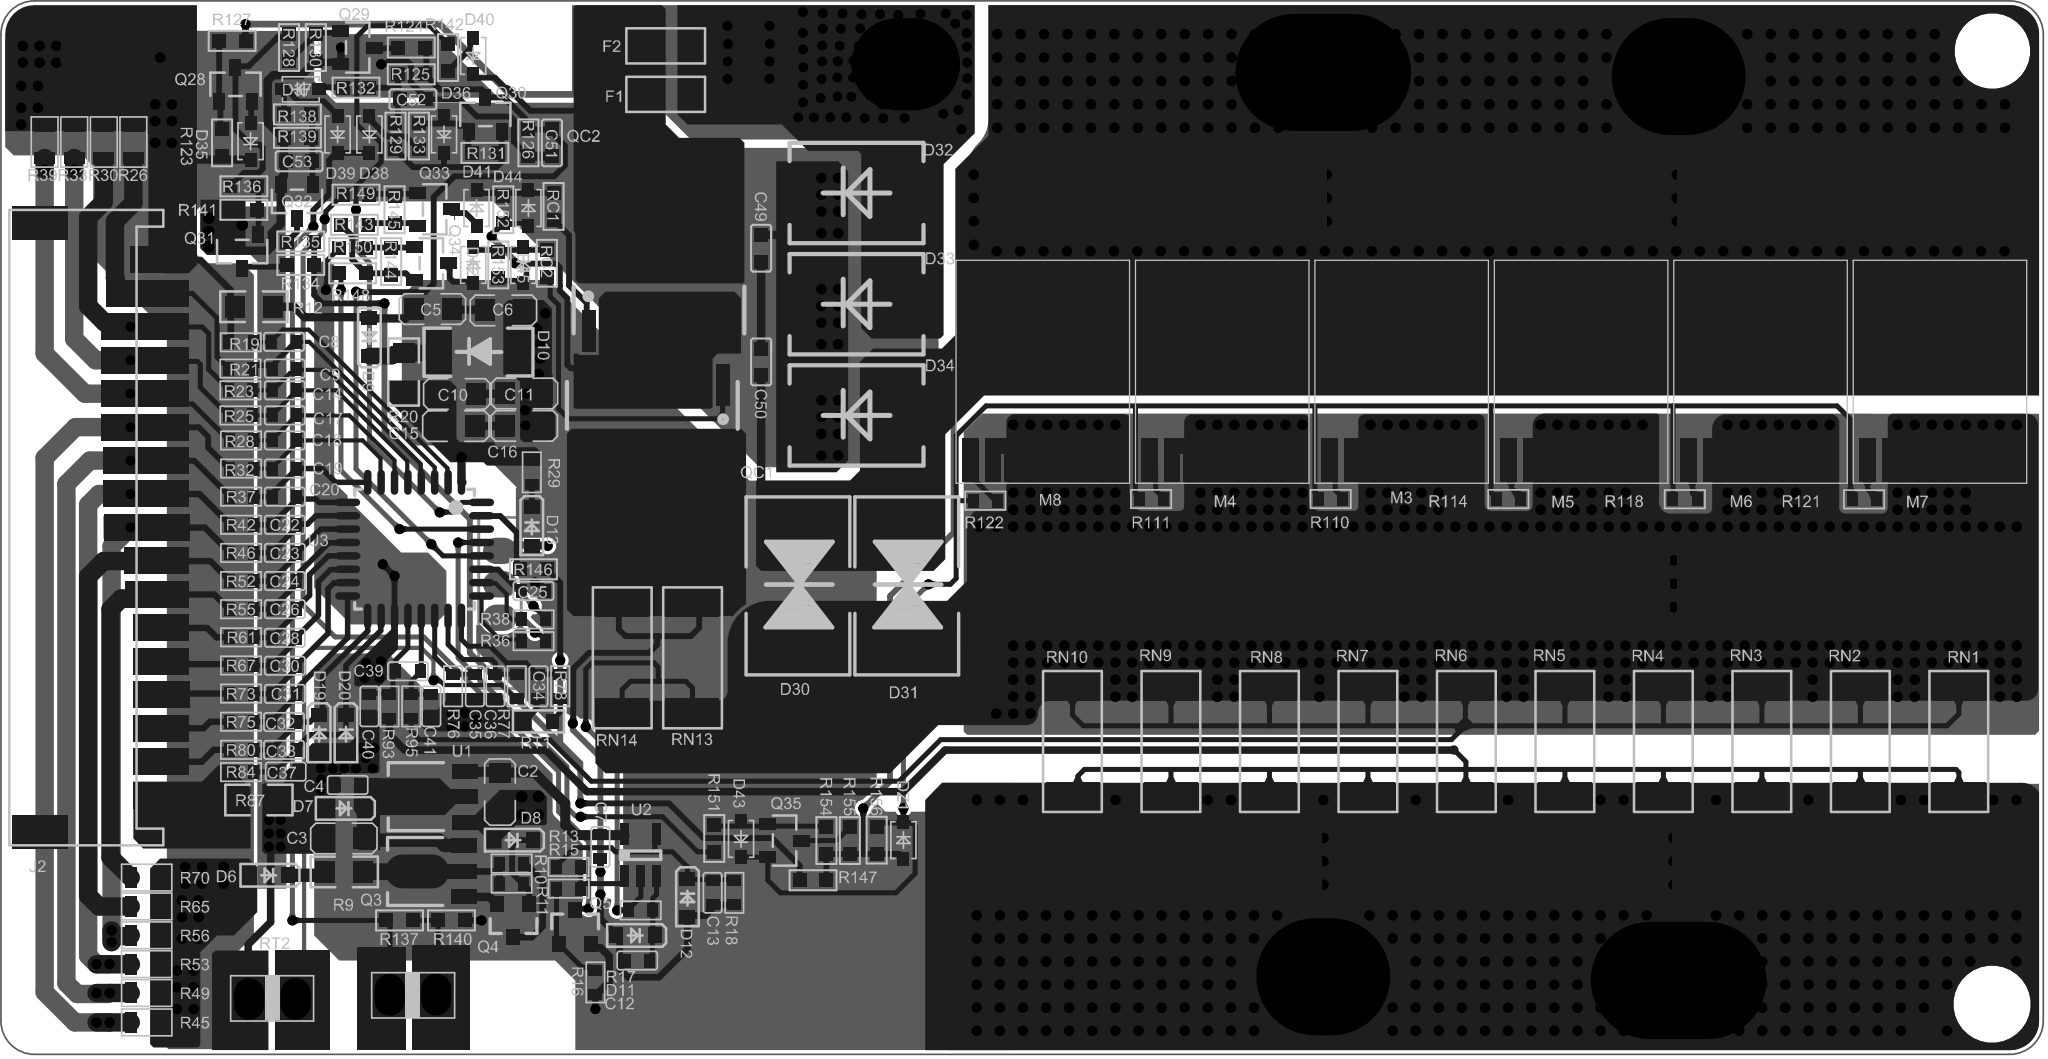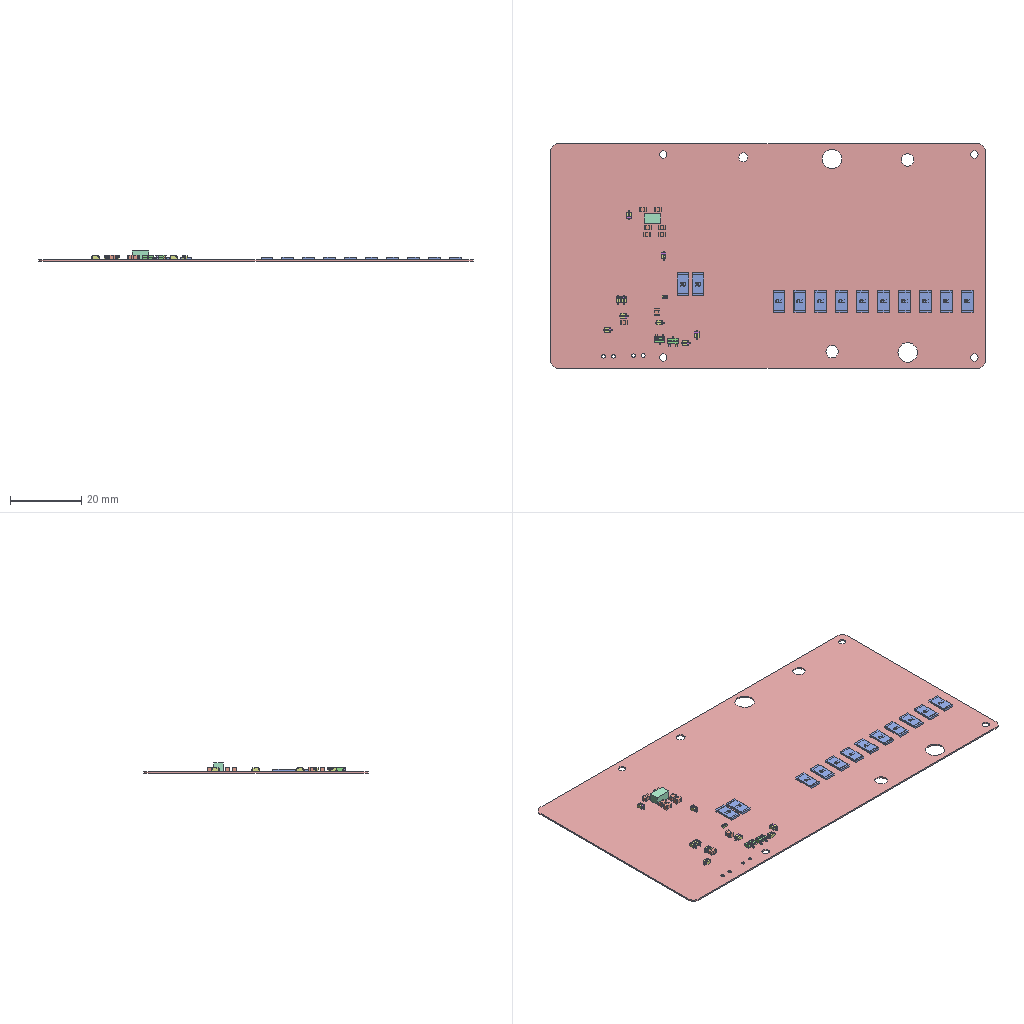Circuit board layout | Altium Designer | box 122 x 63 x 2.8 mm
Layer stack:
# Altium Designer layer stack of  (unit mm; dielectric type: 0 none, 1 core, 2 prepreg, 3 surface material)
index,name,kind,layer,copper_thickness_mm,dielectric_type,dielectric_thickness_mm,dielectric_material,dielectric_constant
0,Top Paste,other,,,,,,
1,Top Overlay,other,,,,,,
2,Top Solder,dielectric,,,3,0.0102,Solder Resist,3.5
3,Top Layer,copper,Top Layer,0.0356,,,,
4,Dielectric 1,dielectric,,,0,0.32,FR-4,4.8
5,Bottom Layer,copper,Bottom Layer,0.0356,,,,
6,Bottom Solder,dielectric,,,3,0.0102,Solder Resist,3.5
7,Bottom Overlay,other,,,,,,
8,Bottom Paste,other,,,,,,
# drill layer pairs: low layer,high layer
drill_pair,Top Layer,Bottom Layer
Part placement:
Designator,Comment,Layer,Footprint,Center-X(mm),Center-Y(mm),Rotation
DZ1,15V,TopLayer,SOD323(A+K-),53.8,12.9,270
R70,0R/NC/16 used in series,TopLayer,R0805A,8.597,10.66,180
R65,0R/NC/17 used in series,TopLayer,R0805A,8.597,8.935,180
R56,0R/NC/16 used in series,TopLayer,R0805A,8.597,7.21,180
R53,0R/NC/17 used in series,TopLayer,R0805A,8.597,5.485,180
Q35,MMBT5401,TopLayer,SOT23-3_BEC,46.708,12.875,270
Q34,MMBT5401,TopLayer,SOT23-3_BEC,25.608,47.4,270
Q33,MMBT5401,TopLayer,SOT23-3_BEC,25.808,50.625,270
Q32,MMBT5551,TopLayer,SOT23-3_BEC,17.575,51.092,180
Q31,MMBT5551,TopLayer,SOT23-3_BEC,14.3,48.092,180
Q30,MMBT5401,TopLayer,SOT23-3_BEC,28.825,56.308,0
Q29,MMBT5551,TopLayer,SOT23-3_BEC,21.208,60.3,270
Q28,MMBT5401,TopLayer,SOT23-3_BEC,13.9,58.108,0
D45,15V,TopLayer,SOD323(A+K-),31.1,47.3,270
D44,15V,TopLayer,SOD323(A+K-),31.4,50.7,270
D43,BAV21WS,TopLayer,SOD323(A+K-),44.1,12.975,90
D42,BAV21WS,TopLayer,SOD323(A+K-),28.1,47.3,270
D41,1N4148WS,TopLayer,SOD323(A+K-),28.3,50.7,270
D40,BAV21WS,TopLayer,SOD323(A+K-),28.1,59.8,90
D39,1N4148WS,TopLayer,SOD323(A+K-),20,55.1,90
D38,1N4148WS,TopLayer,SOD323(A+K-),21.9,55.1,90
D37,1N4148WS,TopLayer,SOD323(A+K-),17.8,57.8,0
D36,5.6V,TopLayer,SOD323(A+K-),26.357,55.106,90
D35,15V,TopLayer,SOD323(A+K-),14.8,54.7,90
F2,40A/72V,TopLayer,R1206L,39.6,60.4,0
F1,5A/125VAC,TopLayer,R1206L,39.6,57.5,0
C53,0.1uF,TopLayer,C0603A,17.7,53.5,0
C52,0.1uF,TopLayer,C0603A,24.5,57.2,180
C51,0.1uF,TopLayer,C0603A,32.8,54.6,90
C50,0.1uF,TopLayer,C0603A,45.3,41.5,90
C49,0.1uF,TopLayer,C0603A,45.3,48.3,90
RC2,100R,TopLayer,R0603A,32.5,47.4,90
RC1,100R,TopLayer,R0603A,32.9,50.8,270
R156,10M,TopLayer,R0603A,52.2,12.9,90
R155,1K,TopLayer,R0603A,50.6,12.875,270
R154,4.7M,TopLayer,R0603A,49.2,12.875,90
R153,1M,TopLayer,R0603A,29.6,47.3,90
R152,1M,TopLayer,R0603A,29.9,50.6,270
R151,1K,TopLayer,R0603A,42.5,13,270
R150,3M,TopLayer,R0603A,20.9,48.3,180
R149,3M,TopLayer,R0603A,21.1,51.5,0
R148,1K,TopLayer,R0603A,20.9,46.8,180
R147,1M,TopLayer,R0603A,48.4,10.5,180
R146,100K,TopLayer,R0603A,31.7,29.1,180
R145,1M,TopLayer,R0603A,23.4,50.6,270
R144,1M,TopLayer,R0603A,23.2,47.5,270
R143,10K,TopLayer,R0603A,21,49.7,180
R142,3M,TopLayer,R0603A,26.6,59.7,90
R141,100K,TopLayer,R0603A,14.4,50.6,0
R140,10K,TopLayer,R0603A,26.8,8.1,0
R139,200K,TopLayer,R0603A,17.6,54.9,0
R138,150K,TopLayer,R0603A,17.6,56.3,180
R137,0Ω/NC,TopLayer,R0603A,23.7,8.1,0
R136,510K,TopLayer,R0603A,14.4,52,180
R135,1K,TopLayer,R0603A,17.8,48.7,0
R134,1K,TopLayer,R0603A,17.8,47.3,0
R133,680K,TopLayer,R0603A,24.857,55.006,270
R132,470K,TopLayer,R0603A,21.1,57.9,180
R131,150K,TopLayer,R0603A,28.8,54,0
R130,100K,TopLayer,R0603A,18.7,60.3,90
R129,200K,TopLayer,R0603A,23.457,55.006,90
R128,510K,TopLayer,R0603A,17.1,60.3,90
R127,100K,TopLayer,R0603A,13.7,60.7,180
R126,10M,TopLayer,R0603A,31.4,54.6,90
R125,NC,TopLayer,R0603A,24.4,58.7,180
R124,1K,TopLayer,R0603A,24.4,60.3,0
R123,20K,TopLayer,R0603A,13.1,54.6,270
S1,SW-SPST,TopLayer,NTC-DIP,24.5,3.654,0
QC2,N MOS*,TopLayer,TOLL,39.2,46.75,0
QC1,N MOS*,TopLayer,TOLL,38.8,36.75,180
D34,RS5M,TopLayer,SMC_MDO-214AB),51,38.3,180
D33,RS5M,TopLayer,SMC_MDO-214AB),51,44.95,180
D32,RS5M,TopLayer,SMC_MDO-214AB),51,51.6,180
C-1,Pth,TopLayer,4*3,53.94,59.3,0
RN14,2mR,TopLayer,R2512A,37,23.8,270
RN9,2mR,TopLayer,R2512A,69.783,18.802,90
RN7,2mR,TopLayer,R2512A,81.549,18.802,90
RN6,2mR,TopLayer,R2512A,87.432,18.802,90
RN5,2mR,TopLayer,R2512A,93.315,18.802,90
RN4,2mR,TopLayer,R2512A,99.198,18.802,90
RN3,2mR,TopLayer,R2512A,105.081,18.802,90
RN2,2mR,TopLayer,R2512A,110.964,18.802,90
R122,100R,TopLayer,R0603m,58.7,33.2,0
R111,100R,TopLayer,R0603m,68.6,33.3,0
R110,100R,TopLayer,R0603m,79.325,33.3,0
M8,SP012N02AGHTO,TopLayer,TOLL,62.05,39.712,0
M4,SP012N02AGHTO,TopLayer,TOLL,72.768,39.712,0
M3,SP012N02AGHTO,TopLayer,TOLL,83.487,39.712,0
R49,0R/NC/16 used in series,TopLayer,R0805A,8.597,3.76,180
R45,0R/NC/17 used in series,TopLayer,R0805A,8.6,2,180
R39,0R/NC/16 used in series,TopLayer,R0805A,2.5,54.65,270
R33,0R/NC/17 used in series,TopLayer,R0805A,4.267,54.65,270
R30,0R/NC/16 used in series,TopLayer,R0805A,6.033,54.65,270
R26,0R/NC/17 used in series,TopLayer,R0805A,7.8,54.65,270
C9,0.1uF,TopLayer,C0603M,16.845,41.1,0
C8,0.1uF,TopLayer,C0603M,16.8,42.7,0
D30,SMDJ150CA,TopLayer,SMC-BI,47.5,28.1,90
D31,SMDJ150CA,TopLayer,SMC-BI,54,28.1,90
J2,PH-2.0mm-17P right-angle connector without latch,TopLayer,HY2.0WT-17A/P_ÎÔÌù´ø¿ÛÄÍÎÂ260¡æ,5.965,31.59,90
C14,0.1uF,TopLayer,C0603M,16.847,39.8,0
C17,0.1uF,TopLayer,C0603M,16.847,38.3,0
C18,0.1uF,TopLayer,C0603M,16.847,36.806,0
C19,0.1uF,TopLayer,C0603M,16.847,35.123,0
R23,510R,TopLayer,R0603m,14.2,39.8,0
R25,510R,TopLayer,R0603m,14.2,38.3,0
R28,510R,TopLayer,R0603m,14.239,36.806,0
R32,510R,TopLayer,R0603m,14.239,35.123,0
RN1,2mR,TopLayer,R2512A,116.847,18.802,90
U3,SH3676014B,TopLayer,LQFP-32,24.6,30.3,180
U2,TP2121-TR,TopLayer,SOT23-5,38.1,12,0
U1,ME6239A50PG,TopLayer,SO-89,26.2,15.5,90
RT2,10K 3435,TopLayer,NTC-DIP,16.102,3.402,180
RT1,10K,TopLayer,R0603,32,20,180
RN10,2mR,TopLayer,R2512A,63.9,18.802,90
RN8,2mR,TopLayer,R2512A,75.666,18.802,90
RN13,10mR,TopLayer,R2512A,41.2,23.8,270
R121,100R,TopLayer,R0603m,111.19,33.28,0
R118,100R,TopLayer,R0603m,100.48,33.29,0
R114,100R,TopLayer,R0603m,89.94,33.3,0
R95,10R,TopLayer,R0603m,24.4,20.9,90
R93,10R,TopLayer,R0603m,23.1,20.9,90
R87,51R,TopLayer,R0805,15.3,15.3,180
R84,510R,TopLayer,R0603m,14.239,16.97,0
R80,510R,TopLayer,R0603m,14.239,18.302,0
R78,1.25K 1%,TopLayer,R0603m,33.3,22.1,270
R77,10R,TopLayer,R0603m,30.7,22.1,270
R76,10K,TopLayer,R0603m,26.9,22.1,270
R75,510R,TopLayer,R0603m,14.239,19.984,0
R73,510R,TopLayer,R0603m,14.239,21.666,0
R67,510R,TopLayer,R0603m,14.239,23.348,0
R61,510R,TopLayer,R0603m,14.239,25.03,0
R55,510R,TopLayer,R0603m,14.239,26.713,0
R52,510R,TopLayer,R0603m,14.239,28.395,0
R46,510R,TopLayer,R0603m,14.239,30.077,0
R42,510R,TopLayer,R0603m,14.239,31.759,0
R38,100R,TopLayer,R0603m,31.7,26.1,180
R37,510R,TopLayer,R0603m,14.239,33.441,0
R36,100R,TopLayer,R0603m,31.7,24.8,180
R29,100R,TopLayer,R0603m,31.6,34.9,90
R20,100R,TopLayer,R0805,23.942,40.895,90
R18,1K 1%,TopLayer,R0603m,43.7,9.753,90
R17,1K 1%,TopLayer,R0603m,38.1,8.7,180
R12,1K,TopLayer,R0805,15,44.8,0
R16,1M,TopLayer,R0603m,35.4,4.4,90
R15,100K 1%,TopLayer,R0603m,33.8,10,180
R13,470K 1%,TopLayer,R0603m,33.8,11.3,0
R11,3M,TopLayer,R0603m,30.4,10.3,0
R10,100K,TopLayer,R0603m,30.4,11.5,0
R9,200R,TopLayer,R0805,20.4,11,180
R21,510R,TopLayer,R0603m,14.2,41.1,0
R19,510R,TopLayer,R0603m,14.222,42.675,0
Q5,MMBT5551,TopLayer,SOT-23S,34.2,7.7,0
Q4,MMBT5551,TopLayer,SOT-23S,30.5,8.1,180
Q3,DXT5551,TopLayer,SOT-89BCE,26.159,11.028,90
M7,SP012N02AGHTO,TopLayer,TOLL,115.642,39.712,0
M6,SP012N02AGHTO,TopLayer,TOLL,104.923,39.712,0
M5,SP012N02AGHTO,TopLayer,TOLL,94.205,39.712,0
J1,UART_M,BottomLayer,CON4/2.0,29.7,27.2,270
D20,BAT46WS,TopLayer,SOD-323-E,20.5,19.261,90
D19,BAT46WS,TopLayer,SOD-323-E,18.9,19.261,90
D13,BAV21WS,TopLayer,SOD-323-E,31.6,31.65,90
D12,1N4148WS,TopLayer,SOD-323-E,40.9,9.453,90
D11,1N4148WS,TopLayer,SOD-323-E,37.8,7.2,0
D10,SMAJ64A,TopLayer,SMA,28.43,42.09,180
D9,BAV21WS,TopLayer,SOD-323-E,21.9,43,270
D8,15V,TopLayer,SOD-323-E,30.5,12.9,0
D7,15V,TopLayer,SOD-323-E,20.4,14.8,0
D6,1N4148WS,TopLayer,SOD-323-E,15.9,10.8,0
C41,1uF,TopLayer,C0603M,25.6,20.9,270
C40,1uF,TopLayer,C0603M,21.9,20.9,270
C39,102,TopLayer,C0603M,24.2,23,180
C37,1uF,TopLayer,C0603M,16.9,17,0
C36,102,TopLayer,C0603M,29.43,22.1,90
C35,102,TopLayer,C0603M,28.2,22.1,90
C34,102,TopLayer,C0603M,32,22.1,90
C33,0.1uF,TopLayer,C0603M,16.8,18.3,0
C32,0.1uF,TopLayer,C0603M,16.8,19.966,0
C31,0.1uF,TopLayer,C0603M,16.847,21.648,0
C30,0.1uF,TopLayer,C0603M,16.847,23.331,0
C28,0.1uF,TopLayer,C0603M,16.847,25,0
C26,0.1uF,TopLayer,C0603M,16.847,26.713,0
C25,1uF/25V,TopLayer,C0603M,31.7,27.8,0
C24,0.1uF,TopLayer,C0603M,16.847,28.395,0
C23,0.1uF,TopLayer,C0603M,16.847,30.077,0
C22,0.1uF,TopLayer,C0603M,16.847,31.759,0
C20,0.1uF,TopLayer,C0603M,16.847,33.441,0
C16,2.2uF/100V,TopLayer,C0805,31.125,37.672,0
C15,2.2uF/100V,TopLayer,C0805,27.039,37.662,0
C13,0.47uF,TopLayer,C0603M,42.4,9.753,270
C12,0.47uF,TopLayer,C0603M,37.9,5.7,180
C11,0.1uF/100V,TopLayer,C0805,31.135,39.612,0
C10,0.1uF/100V,TopLayer,C0805,27.095,39.582,0
C6,2.2uF/100V,TopLayer,C0805,29.93,44.58,180
C5,2.2uF/100V,TopLayer,C0805,25.69,44.66,180
C7,10nF,TopLayer,C0603M,35.7,12.5,270
C4,0.1uF,TopLayer,C0603M,20.6,16.2,180
C3,2.2uF/50V,TopLayer,C0805,20.4,13,180
C2,10uF/25V,TopLayer,C0805,29.7,15.8,270
Pad and via stacks:
# Altium Designer via and pad stacks of  (unit mm). Each distinct definition once, with the count of objects using it.
# via: kind,start_layer,end_layer,hole_mm,diameter_mm,mode(0 simple;1 top-mid-bottom;2 full stack),diameter_per_layer,count,example_net
# pad: kind,layer,hole_mm,hole_type(0 round;1 square;2 slot),plating,top_size,top_shape(1 round;2 rect;3 octagon;9 rounded rect),mid_size,bottom_size,mode,footprint,size_per_layer,count,example
pad,Top Layer,0,0,plated,1.143x1.27,2,1.143x1.27,1.143x1.27,0,C0805,,16,C16.1
pad,Top Layer,0,0,plated,1.5x2.6,2,1.5x2.6,1.5x2.6,0,SMA,,2,D10.A
pad,Top Layer,0,0,plated,0.8x0.9,2,0.8x0.9,0.8x0.9,0,SOD-323-E,,18,D20.A
pad,Top Layer,0,0,plated,7.45x10.2,2,7.45x10.2,7.45x10.2,0,TOLL,,6,M7.D
pad,Top Layer,0,0,plated,0.9x7,2,0.9x7,0.9x7,0,TOLL,,6,M7.S
pad,Top Layer,0,0,plated,1x2.61,2,1x2.61,1x2.61,0,TOLL,,42,M7.S
pad,Top Layer,0,0,plated,0.9x2.61,2,0.9x2.61,0.9x2.61,0,TOLL,,6,M7.S
pad,Top Layer,0,0,plated,0.8636x1.524,2,0.8636x1.524,0.8636x1.524,0,SOT-89BCE,,2,Q3.B
pad,Top Layer,0,0,plated,0.8636x2.54,2,0.8636x2.54,0.8636x2.54,0,SOT-89BCE,,1,Q3.C
pad,Top Layer,0,0,plated,2.032x3.81,1,2.032x3.81,2.032x3.81,0,SOT-89BCE,,1,Q3.C
pad,Top Layer,0,0,plated,0.9x0.8,2,0.9x0.8,0.9x0.8,0,SOT-23S,,6,Q5.E
pad,Top Layer,0,0,plated,1.143x1.27,2,1.143x1.27,1.143x1.27,0,R0805,,8,R87.2
pad,Top Layer,0,0,plated,0.889x0.762,2,0.889x0.762,0.889x0.762,0,R0603,,2,RT1.2
pad,Top Layer,0,0,plated,2.032x3.81,1,2.032x3.81,2.032x3.81,0,SO-89,,1,U1.2
pad,Top Layer,0,0,plated,0.8636x2.54,2,0.8636x2.54,0.8636x2.54,0,SO-89,,1,U1.2
pad,Top Layer,0,0,plated,0.8636x1.524,2,0.8636x1.524,0.8636x1.524,0,SO-89,,2,U1.3
pad,Top Layer,0,0,plated,1.27x0.508,2,1.27x0.508,1.27x0.508,0,SOT23-5,,5,U2.3
pad,Top Layer,0,0,plated,0.45x1.5,1,0.45x1.5,0.45x1.5,0,LQFP-32,,32,U3.32
pad,Top Layer,0,0,plated,3.175x1.524,2,3.175x1.524,3.175x1.524,0,R2512A,,24,RN1.1
pad,Top Layer,0,0,plated,2.8x1,2,2.8x1,2.8x1,0,HY2.0WT-17A/P \u00CE\u00D4\u00CC\u00F9\u00B4\u00F8\u00BF\u00DB\u00C4\u00CD\u00CE\u00C2260\u00A1\u00E6,,17,J2.13
pad,Top Layer,0,0,plated,3.3x2,2,3.3x2,3.3x2,0,HY2.0WT-17A/P \u00CE\u00D4\u00CC\u00F9\u00B4\u00F8\u00BF\u00DB\u00C4\u00CD\u00CE\u00C2260\u00A1\u00E6,,2,J2.0
pad,Top Layer,0,0,plated,2x3.1,2,2x3.1,2x3.1,0,SMC-BI,,4,D30.K
pad,Top Layer,0,0,plated,0.65x0.8,2,0.65x0.8,0.65x0.8,0,C0603M,,56,C9.1
pad,Top Layer,0,0,plated,0.8x0.65,2,0.8x0.65,0.8x0.65,0,R0603m,,76,R122.1
pad,Top Layer,0,0,plated,1.8x3.2,2,1.8x3.2,1.8x3.2,0,SMC_MDO-214AB),,6,D34.1
pad,Top Layer,0,0,plated,9.9x8,2,9.9x8,9.9x8,0,TOLL,,2,QC2.3
pad,Top Layer,0,0,plated,0.8x8,2,0.8x8,0.8x8,0,TOLL,,2,QC2.2
pad,Top Layer,0,0,plated,1.7x0.8,2,1.7x0.8,1.7x0.8,0,TOLL,,14,QC2.2
pad,Top Layer,0,0,plated,2.5x0.8,2,2.5x0.8,2.5x0.8,0,TOLL,,2,QC2.1
pad,Top Layer,0,0,plated,0.8x0.8,2,0.8x0.8,0.8x0.8,0,R0603A,,72,RC2.2
pad,Top Layer,0,0,plated,0.8x0.8,2,0.8x0.8,0.8x0.8,0,C0603A,,10,C53.1
pad,Top Layer,0,0,plated,0.9x1.6,2,0.9x1.6,0.9x1.6,0,R1206L,,4,F2.1
pad,Top Layer,0,0,plated,0.7x1,2,0.7x1,0.7x1,0,SOT23-3_BEC,,24,Q35.B
pad,Top Layer,0,0,plated,0.7x1.2,2,0.7x1.2,0.7x1.2,0,R0805A,,20,R70.2
pad,Top Layer,0,0,plated,0.8x0.7,2,0.8x0.7,0.8x0.7,0,SOD323(A+K-),,24,DZ1.A
pad,Top Layer,0,0,plated,5x3.5,1,5x3.5,5x3.5,0,,,1,B
pad,Top Layer,0,0,plated,20x5,2,20x5,20x5,0,,,9,32
pad,Top Layer,0,2,plated,1x1,1,1x1,1x1,0,,,2,28
pad,Bottom Layer,0,0,plated,1.575x2.032,1,1.575x2.032,1.575x2.032,0,CON4/2.0,,4,J1.4
pad,Bottom Layer,0,0,plated,20x5,2,20x5,20x5,0,,,9,31
pad,Bottom Layer,0,2,plated,1x1,1,1x1,1x1,0,,,1,29
pad,Multi-Layer,1,0,plated,1.8x2.5,1,1.8x2.5,1.8x2.5,0,NTC-DIP,,4,RT2.1
pad,Multi-Layer,2.5,0,plated,6.5x5.5,1,6.5x5.5,6.5x5.5,0,4*3,,1,C-1.1
pad,Multi-Layer,5.5,0,plated,10.5x7,1,10.5x7,10.5x7,0,,,2,30
pad,Multi-Layer,3.5,0,plated,8x7,1,8x7,8x7,0,,,2,30
via,Top Layer,Bottom Layer,0.4,0.635,0,,11,BC8
via,Top Layer,Bottom Layer,0.381,0.635,0,,846,BC16
via,Top Layer,Bottom Layer,0.4,0.6,0,,133,BC8
via,Top Layer,Bottom Layer,0.5,0.7,0,,8,GND
Copper pours:
name,layer,net,type(0 solid;1 hatched;2 none)
NONET_L02_P-001,Top Layer,BC16,0
NONET_L02_P-001,Top Layer,BC0,0
NONET_L02_P-001,Top Layer,BC16,0
NONET_L02_P-001,Top Layer,CHGD1,0
NONET_L02_P-001,Top Layer,NetD44_A,0
NONET_L02_P-001,Top Layer,GND,0
NONET_L02_P-001,Top Layer,GND,0
NONET_L02_P-001,Top Layer,GND,0
NONET_L02_P-001,Top Layer,GND,0
NONET_L02_P-001,Top Layer,NetR77_2,0
NONET_L02_P-001,Top Layer,GND,0
NONET_L02_P-001,Top Layer,C-,0
NONET_L02_P-001,Top Layer,GND,0
NONET_L02_P-001,Top Layer,VBAT_M,0
NONET_L02_P-001,Top Layer,GND,0
NONET_L02_P-001,Top Layer,NetR137_2,0
NONET_L02_P-001,Top Layer,NetD38_K,0
NONET_L02_P-001,Top Layer,GND1,0
NONET_L02_P-001,Top Layer,BC16,0
NONET_L02_P-001,Top Layer,DSGD1,0
NONET_L02_P-001,Top Layer,NetC3_1,0
NONET_L01_P-001,Top Layer,DG-,0
NONET_L02_P-001,Top Layer,GND,0
NONET_L02_P-001,Bottom Layer,GND,0
NONET_L02_P-001,Bottom Layer,GND,0
BC7_L02_P217,Bottom Layer,BC7,0
BC8_L02_P242,Bottom Layer,BC8,0
BC9_L02_P241,Bottom Layer,BC9,0
NONET_L02_P-001,Bottom Layer,BC16,0
NONET_L02_P-001,Bottom Layer,GND,0
BC11_L02_P197,Bottom Layer,BC11,0
BC12_L02_P196,Bottom Layer,BC12,0
BC13_L02_P195,Bottom Layer,BC13,0
BC14_L02_P194,Bottom Layer,BC14,0
NONET_L02_P-001,Bottom Layer,GND,0
NONET_L02_P-001,Bottom Layer,DSGD1,0
C-_L02_P104,Bottom Layer,C-,0
BC10_L02_P198,Bottom Layer,BC10,0
NONET_L02_P-001,Bottom Layer,DG-,0
Bottom Layer-GND,Bottom Layer,GND,0
Design rules, without the lines most boards share:
# Altium Designer design rules of  (exported by Altium Designer, unit mm)
# columns: name | kind | enabled | priority | scope1 | scope2 | descriptor | typed fields (field=value)
Schematic Supply Nets_2 | 41 | enabled | 1 | InNet('DSGD1') | All | Supply Net(s)(InNet('DSGD1')) |
Schematic Supply Nets_5 | 41 | enabled | 2 | InNet('C-') | All | Supply Net(s)(InNet('C-')) |
Schematic Supply Nets | 41 | enabled | 3 | InNet('BC16') | All | Supply Net(s)(InNet('BC16')) |
Schematic Supply Nets_6 | 41 | enabled | 4 | InNet('GND1') | All | Supply Net(s)(InNet('GND1')) |
Schematic Supply Nets_4 | 41 | enabled | 5 | InNet('5V') | All | Supply Net(s)(InNet('5V')) |
Schematic Supply Nets_3 | 41 | enabled | 6 | InNet('GND') | All | Supply Net(s)(InNet('GND')) |
NetAntennae | 56 | enabled | 1 | All | All | Net Antennae (Tolerance=0mm) (All) |
SilkToSilkClearance | 55 | disabled | 1 | All | All | Silk to Silk (Clearance=0mm) (Disabled)(All),(All) |
SilkToSolderMaskClearance | 54 | disabled | 1 | IsPad | All | Silk To Solder Mask (Clearance=0mm) (Disabled)(IsPad),(All) |
MinimumSolderMaskSliver | 53 | disabled | 1 | All | All | Minimum Solder Mask Sliver (Gap=0mm) (Disabled)(All),(All) |
HoleToHoleClearance | 52 | disabled | 1 | All | All | Hole To Hole Clearance (Gap=0mm) (Disabled)(All),(All) | gap=0
DiffPairsRouting | 51 | enabled | 1 | All | All | Differential Pairs Uncoupled Length using the Gap Constraints (Min=0.254mm) (Max=0.254mm) (Prefered=0.254mm)  and Width Constraints (Min=0.381mm) (Max=0.381mm) (Prefered=0.381mm) (All) |
HoleSize | 42 | enabled | 1 | All | All | Hole Size Constraint (Min=0.025mm) (Max=10mm) (All) |
Height | 50 | disabled | 1 | All | All | Height Constraint (Min=0mm) (Max=25.4mm) (Prefered=12.7mm) (Disabled)(All) | min_height=0 max_height=25.4
ComponentClearance | 24 | disabled | 1 | All | All | Component Clearance Constraint ( Horizontal Gap = 0.254mm, Vertical Gap = 0.254mm ) (Disabled)(All),(All)  | gap=0.254
SolderMaskExpansion | 13 | enabled | 1 | All | All | Solder Mask Expansion (Expansion =0.102mm) (All) | expansion=0.1016
PasteMaskExpansion | 14 | enabled | 1 | All | All | Paste Mask Expansion (Expansion =0mm) (All) | expansion=0
RoutingVias | 11 | enabled | 1 | All | All | Routing Via (MinHoleWidth=0.4mm) (MaxHoleWidth=0.711mm) (PreferredHoleWidth=0.5mm) (MinWidth=0.6mm) (MaxWidth=1.27mm) (PreferedWidth=0.8mm) (All) | via_min_hole=0.4 via_max_hole=0.7112 via_preferred_diameter=0.8 via_preferred_hole=0.5
RoutingCorners | 10 | enabled | 1 | All | All | Routing Corners (Style=45-Degree) (Min Setback=2.54mm) (Max Setback=2.54mm) (All) |
Width | 2 | enabled | 1 | All | All | Width Constraint (Min=0.2mm) (Max=20mm) (Preferred=0.3mm) (All) |
PolygonConnect | 20 | enabled | 1 | All | All | Polygon Connect Rule(Direct Connect )(Conductor Width=0.254mm) (Relief Angle=90 Angle) (Entries=4) (Air Gap Width=0.254mm) (All),(All) | connect_style(0=relief,1=direct,2=none)=1 relief_conductor_width=0.254 relief_entries=4
PlaneClearance | 12 | enabled | 1 | All | All | Power Plane Clearance (Clearance =0.508mm) (All) | clearance=0.508
PlaneConnect | 6 | enabled | 1 | All | All | Power Plane Connect Rule(Relief Connect )(Expansion=0.508mm) (Conductor Width=0.254mm) (Air Gap=0.254mm) (Entries=4) (All) | relief_conductor_width=0.254 relief_entries=4 relief_expansion=0.508
Clearance | 0 | enabled | 1 | All | All | Clearance Constraint (Gap=0.2mm) (All),(All) | gap=0.2
Classes set for this board:
# Altium Designer classes of  (member kind: 0 net, 1 component, 2 from-to, 3 pad, 4 layer, 5 differential pair, 6 design channel, 7 polygon, 8 structure, 9 xSignal)
# columns: class name | member kind | superclass | members
B-1024-JZ02 V0   0915 | 1 | no | M5; M6; M7; RN1; M3; M4; M8; RN2; RN3; RN4; RN5; R25; R18; D7; D9; D11; D19; R73; R76; R28; R78; R80; RT2; U2; C25; C31; Q3; Q5; R19; R21; R10; R11; C2; C3; C4; C5; C6; C7; C8; C9; C10; C11; C12; C13; C14; C15; C16; C17; C18; C19; C20; C22; C23; C24; C26; C28; C30; C32; C33; C34; C35; C36; C37; C39; C40; C41; D6; D8; D10; D12; D13; D20; D30; D31; J1; J2; Q4; R9; R12; R13; R15; R16; R17; R20; R23; R26; R29; R30; R32; R33; R36; R37; R38; R39; R42; R45; R46; R49; R52; R55; R61; R67; R75; R77; R84; R87; R93; R95; R110; R111; R114; R118; R121; R122; RT1; U1; U3; RN6; RN8; RN7; RN9; RN10; RN13; RN14; C-1; D32; D33; D34; QC1; QC2; S1; R123; R124; R125; R126; R127; R128; R129; R130; R131; R132; R133; R134; R135; R136; R137; R138; R139; R140; R141; R142; R143; R144; R145; R146; R147; R148; R149; R150; R151; R152; R153; R154; R155; R156; RC1; RC2; C49; C50; C51; C52; C53; F1; F2; D35; D36; D37; D38; D39; D40; D41; D42; D43; D44; D45; Q28; Q29; Q30; Q31; Q32; Q33; Q34; Q35; R53; R56; R65; R70; DZ1;